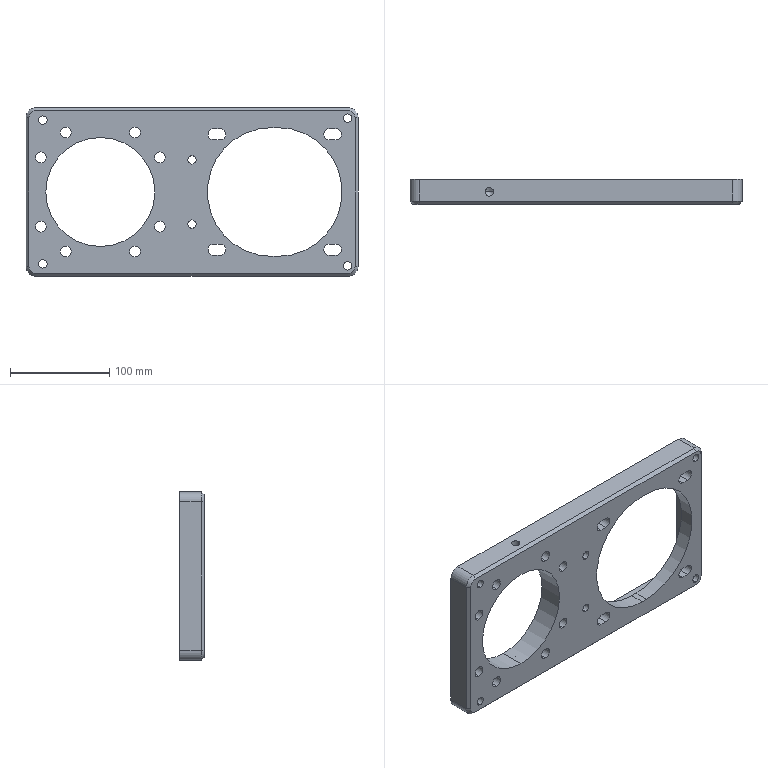Part | SolidWorks | features HoleWzd 9, ICE 4, MoveFace 4, MirrorPattern 3, Chamfer 1, Extrusion 1, Fillet 1 | 1 solid | 113 faces | box 335 x 25 x 170 mm | volume 717401 mm3 | cylinder 72 | plane 33 | cone 8 | commonest cylinder face diameters 11 x24 8.5 x16 18 x16 5.5 x4 15 x4 20 x4